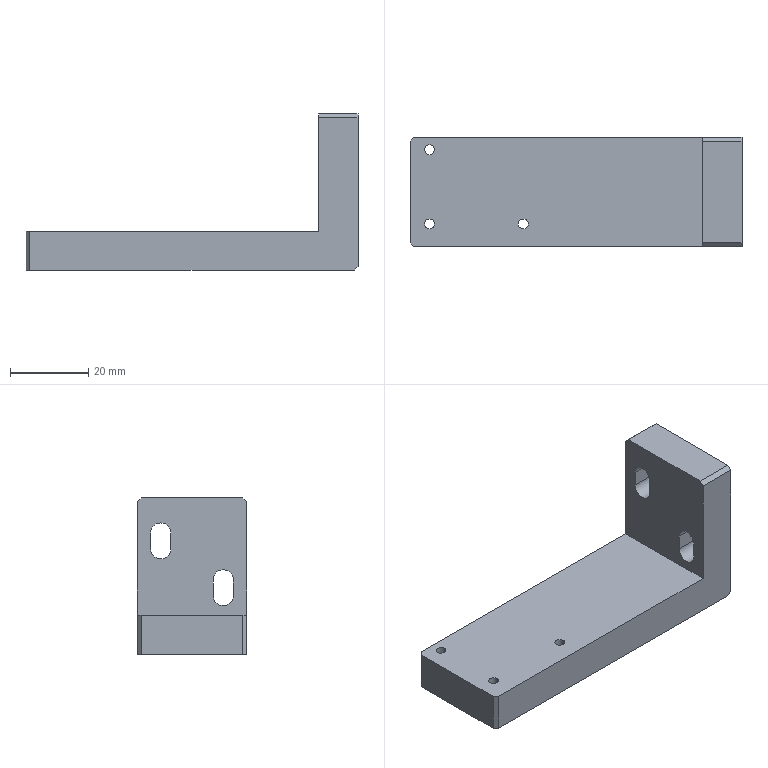Part | STEP file | cylinder fixing plate 2 | 1 solid | 29 faces | box 85 x 28 x 40 mm | volume 31178 mm3 | plane 17 | cylinder 12 | commonest cylinder face diameters 2.5 x6 5.2 x6